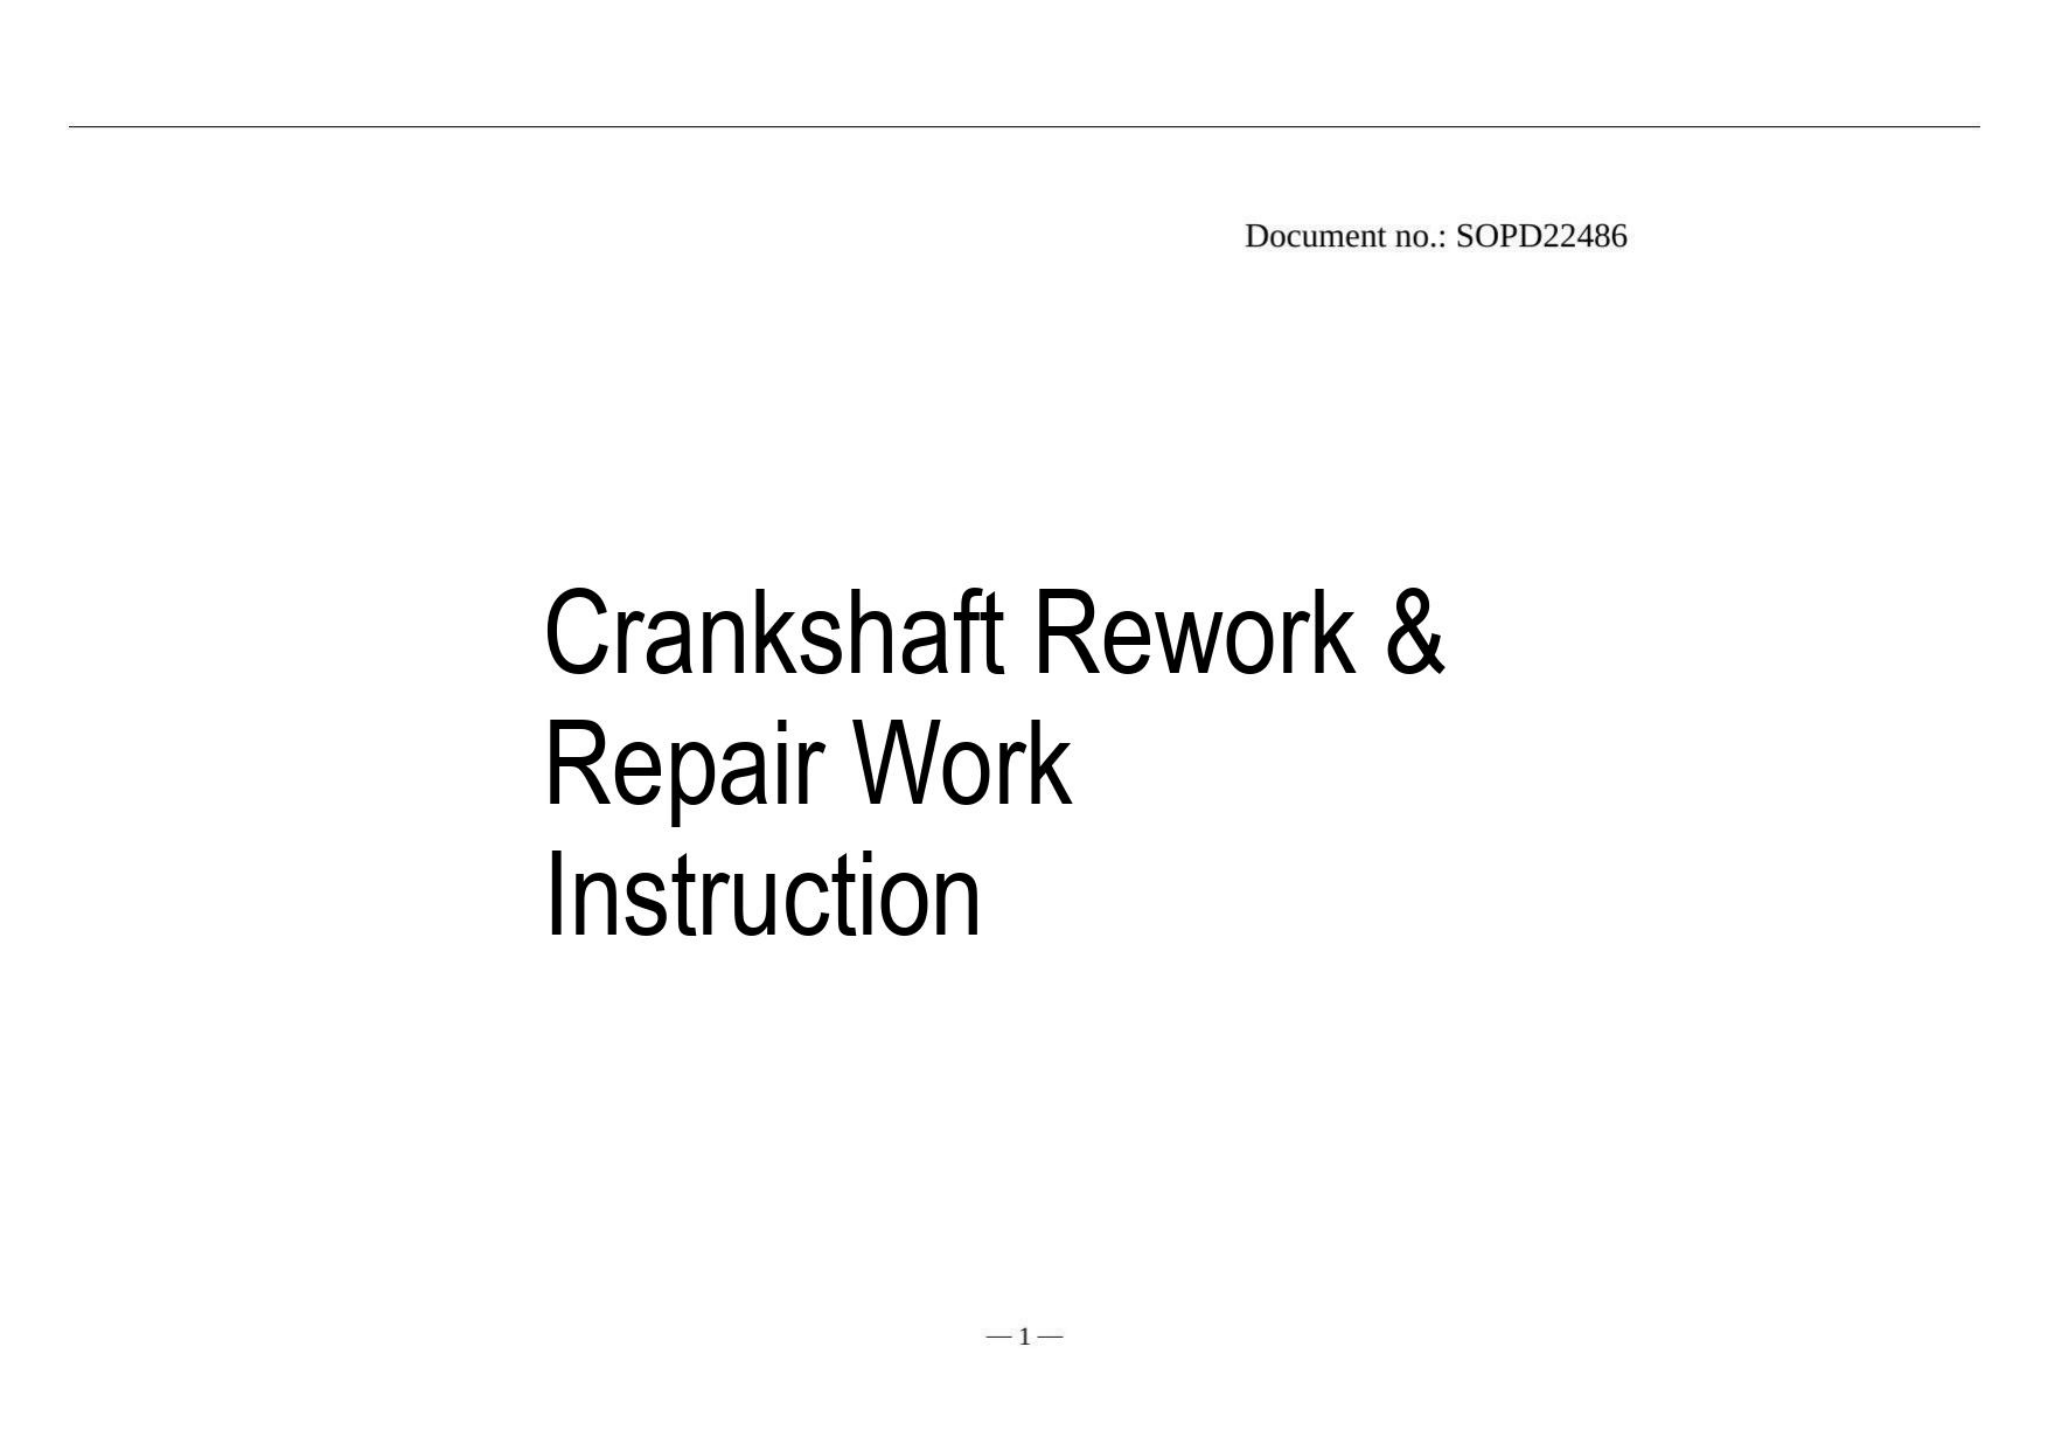Document no.: SOPD22486

Crankshaft Rework & Repair Work Instruction

—1—
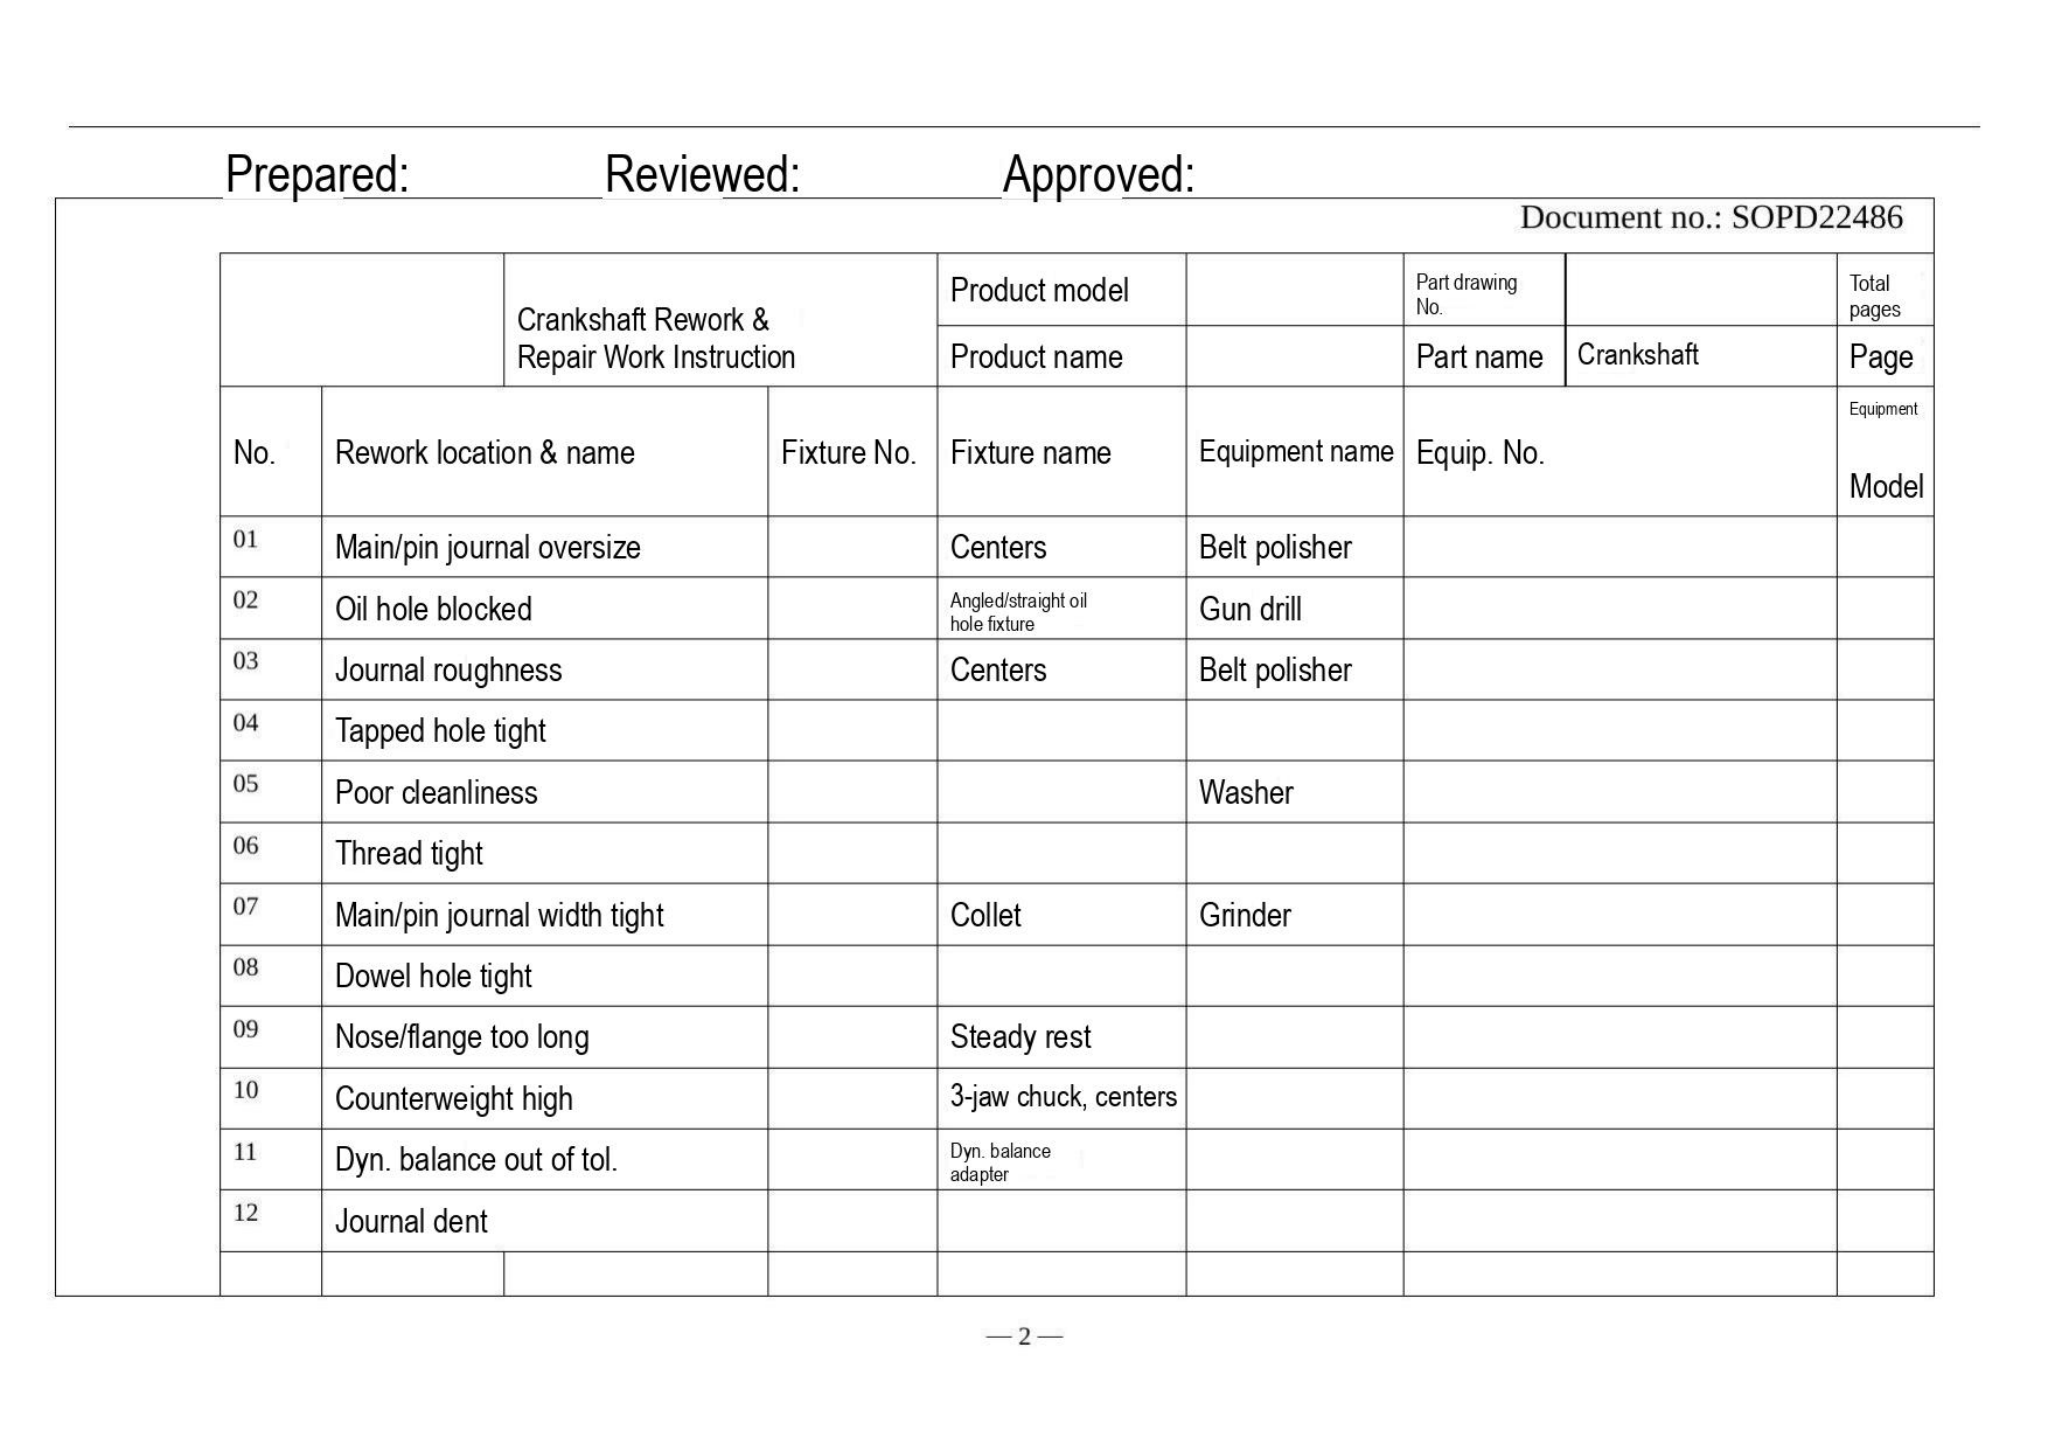Prepared: Reviewed: Approved:

Document no.: SOPD22486

| | Crankshaft Rework & Repair Work Instruction | Product model | | Part drawing No. | | Total pages |
|---|---|---|---|---|---|---|
| | | Product name | | Part name | Crankshaft | Page |

| No. | Rework location & name | Fixture No. | Fixture name | Equipment name | Equip. No. | Equipment Model |
|---|---|---|---|---|---|---|
| 01 | Main/pin journal oversize | | Centers | Belt polisher | | |
| 02 | Oil hole blocked | | Angled/straight oil hole fixture | Gun drill | | |
| 03 | Journal roughness | | Centers | Belt polisher | | |
| 04 | Tapped hole tight | | | | | |
| 05 | Poor cleanliness | | | Washer | | |
| 06 | Thread tight | | | | | |
| 07 | Main/pin journal width tight | | Collet | Grinder | | |
| 08 | Dowel hole tight | | | | | |
| 09 | Nose/flange too long | | Steady rest | | | |
| 10 | Counterweight high | | 3-jaw chuck, centers | | | |
| 11 | Dyn. balance out of tol. | | Dyn. balance adapter | | | |
| 12 | Journal dent | | | | | |
| | | | | | | |

—2—
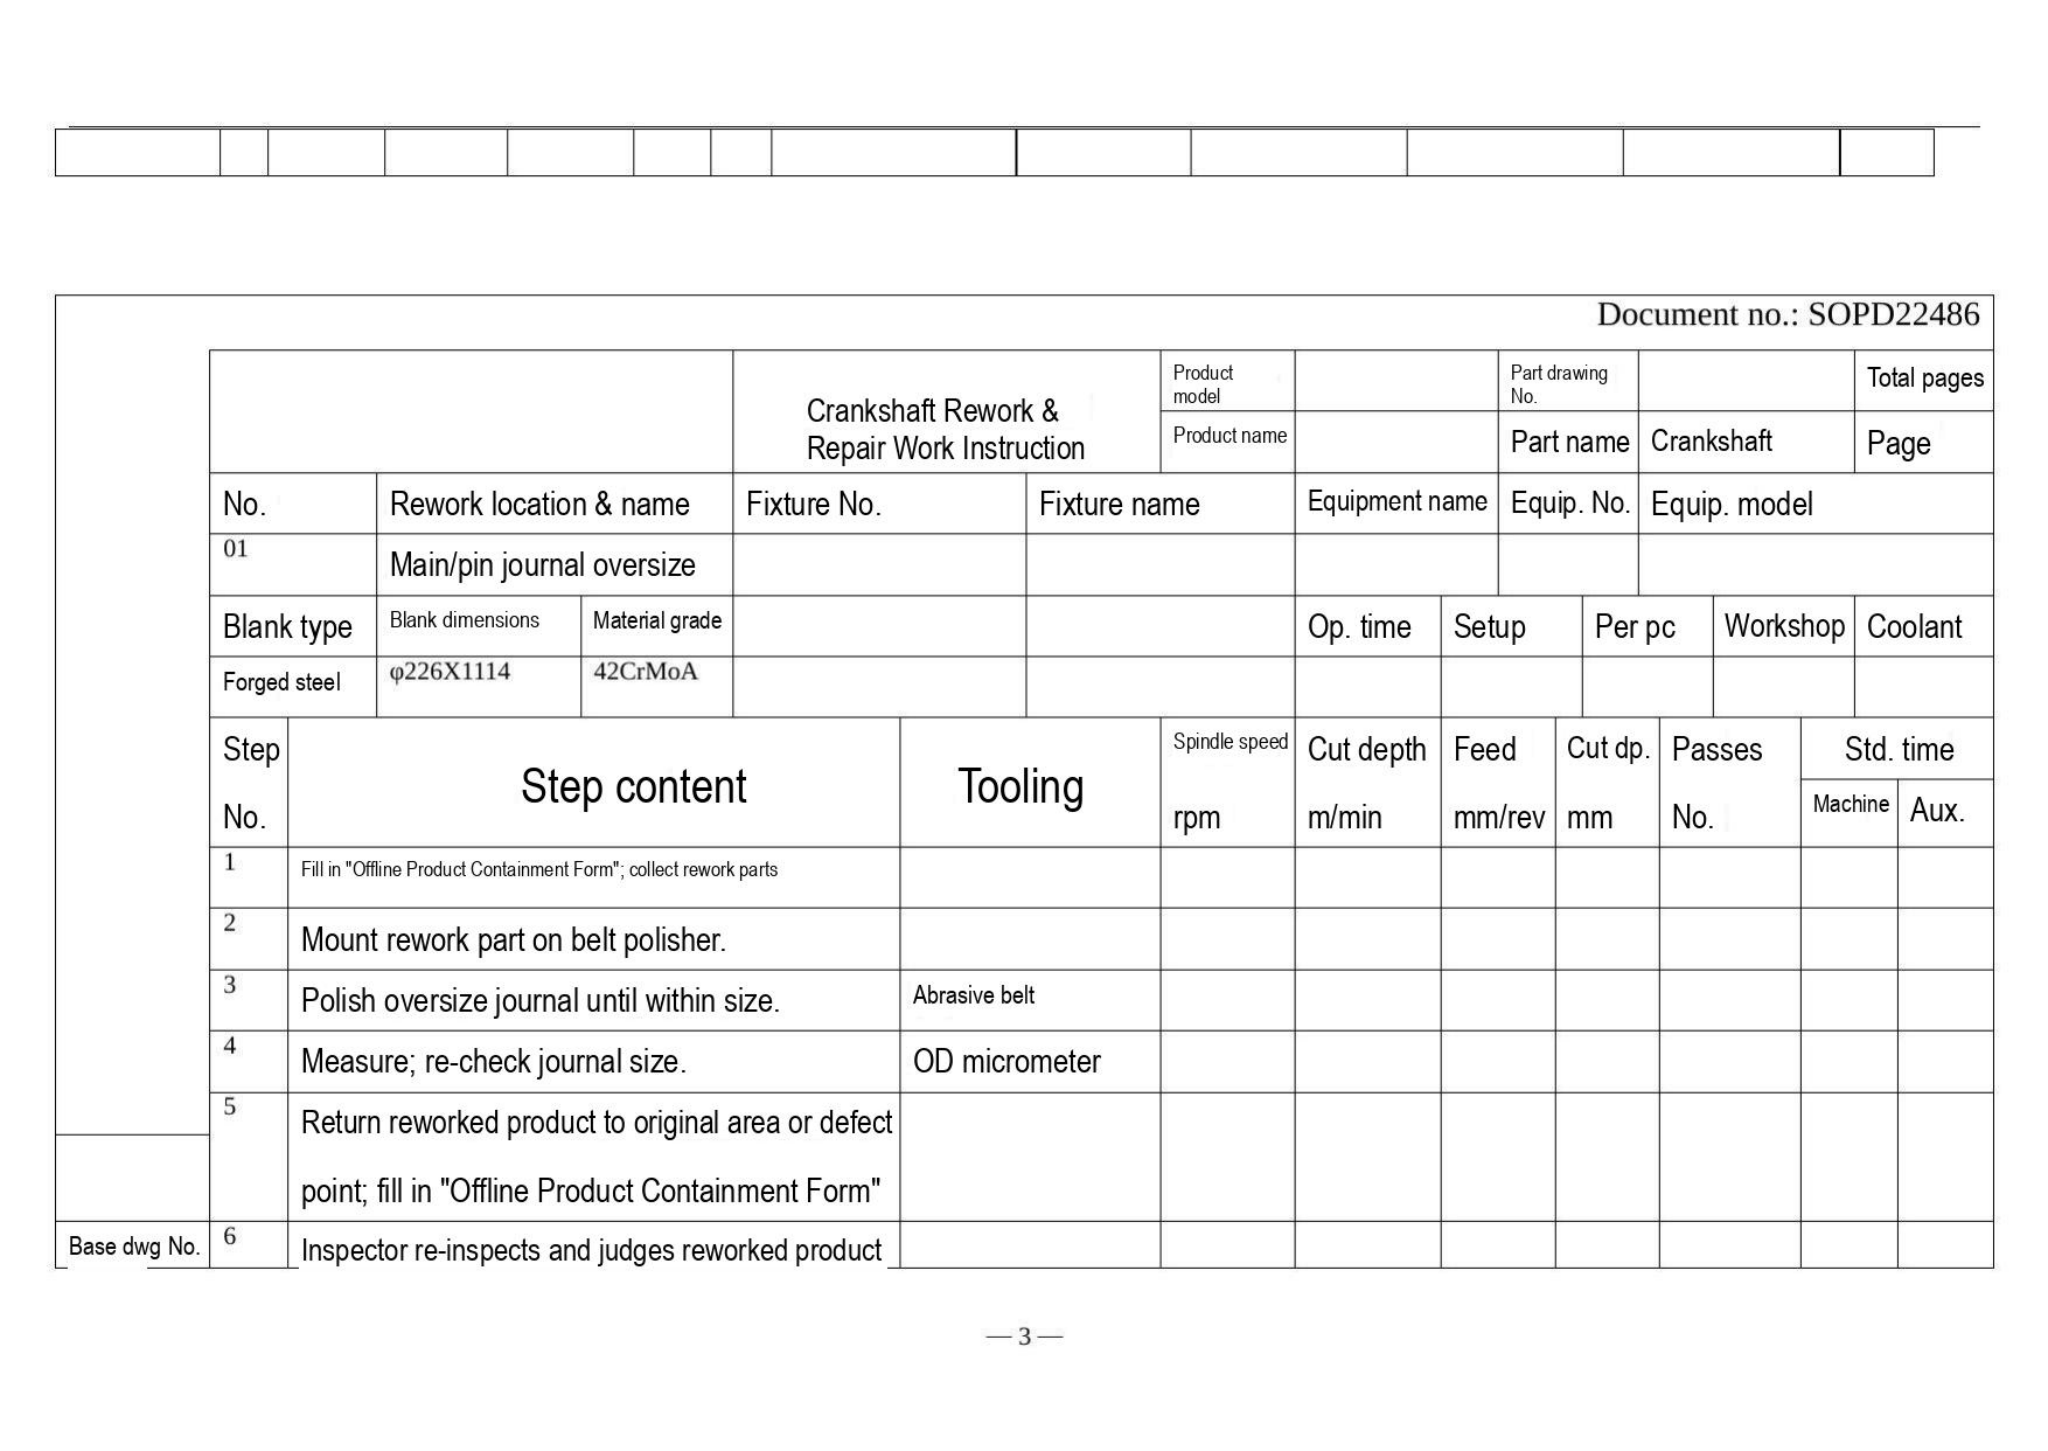Document no.: SOPD22486

| | Crankshaft Rework & Repair Work Instruction | Product model | | Part drawing No. | | Total pages |
|---|---|---|---|---|---|---|
| | | Product name | | Part name | Crankshaft | Page |

| No. | Rework location & name | Fixture No. | Fixture name | Equipment name | Equip. No. | Equip. model |
|---|---|---|---|---|---|---|
| 01 | Main/pin journal oversize | | | | | |

| Blank type | Blank dimensions | Material grade | | | Op. time | Setup | Per pc | Workshop | Coolant |
|---|---|---|---|---|---|---|---|---|---|
| Forged steel | φ226X1114 | 42CrMoA | | | | | | | |

| Step No. | Step content | Tooling | Spindle speed rpm | Cut depth m/min | Feed mm/rev | Cut dp. mm | Passes No. | Std. time Machine | Std. time Aux. |
|---|---|---|---|---|---|---|---|---|---|
| 1 | Fill in "Offline Product Containment Form"; collect rework parts | | | | | | | | |
| 2 | Mount rework part on belt polisher. | | | | | | | | |
| 3 | Polish oversize journal until within size. | Abrasive belt | | | | | | | |
| 4 | Measure; re-check journal size. | OD micrometer | | | | | | | |
| 5 | Return reworked product to original area or defect point; fill in "Offline Product Containment Form" | | | | | | | | |
| 6 | Inspector re-inspects and judges reworked product | | | | | | | | |

Base dwg No.

— 3 —
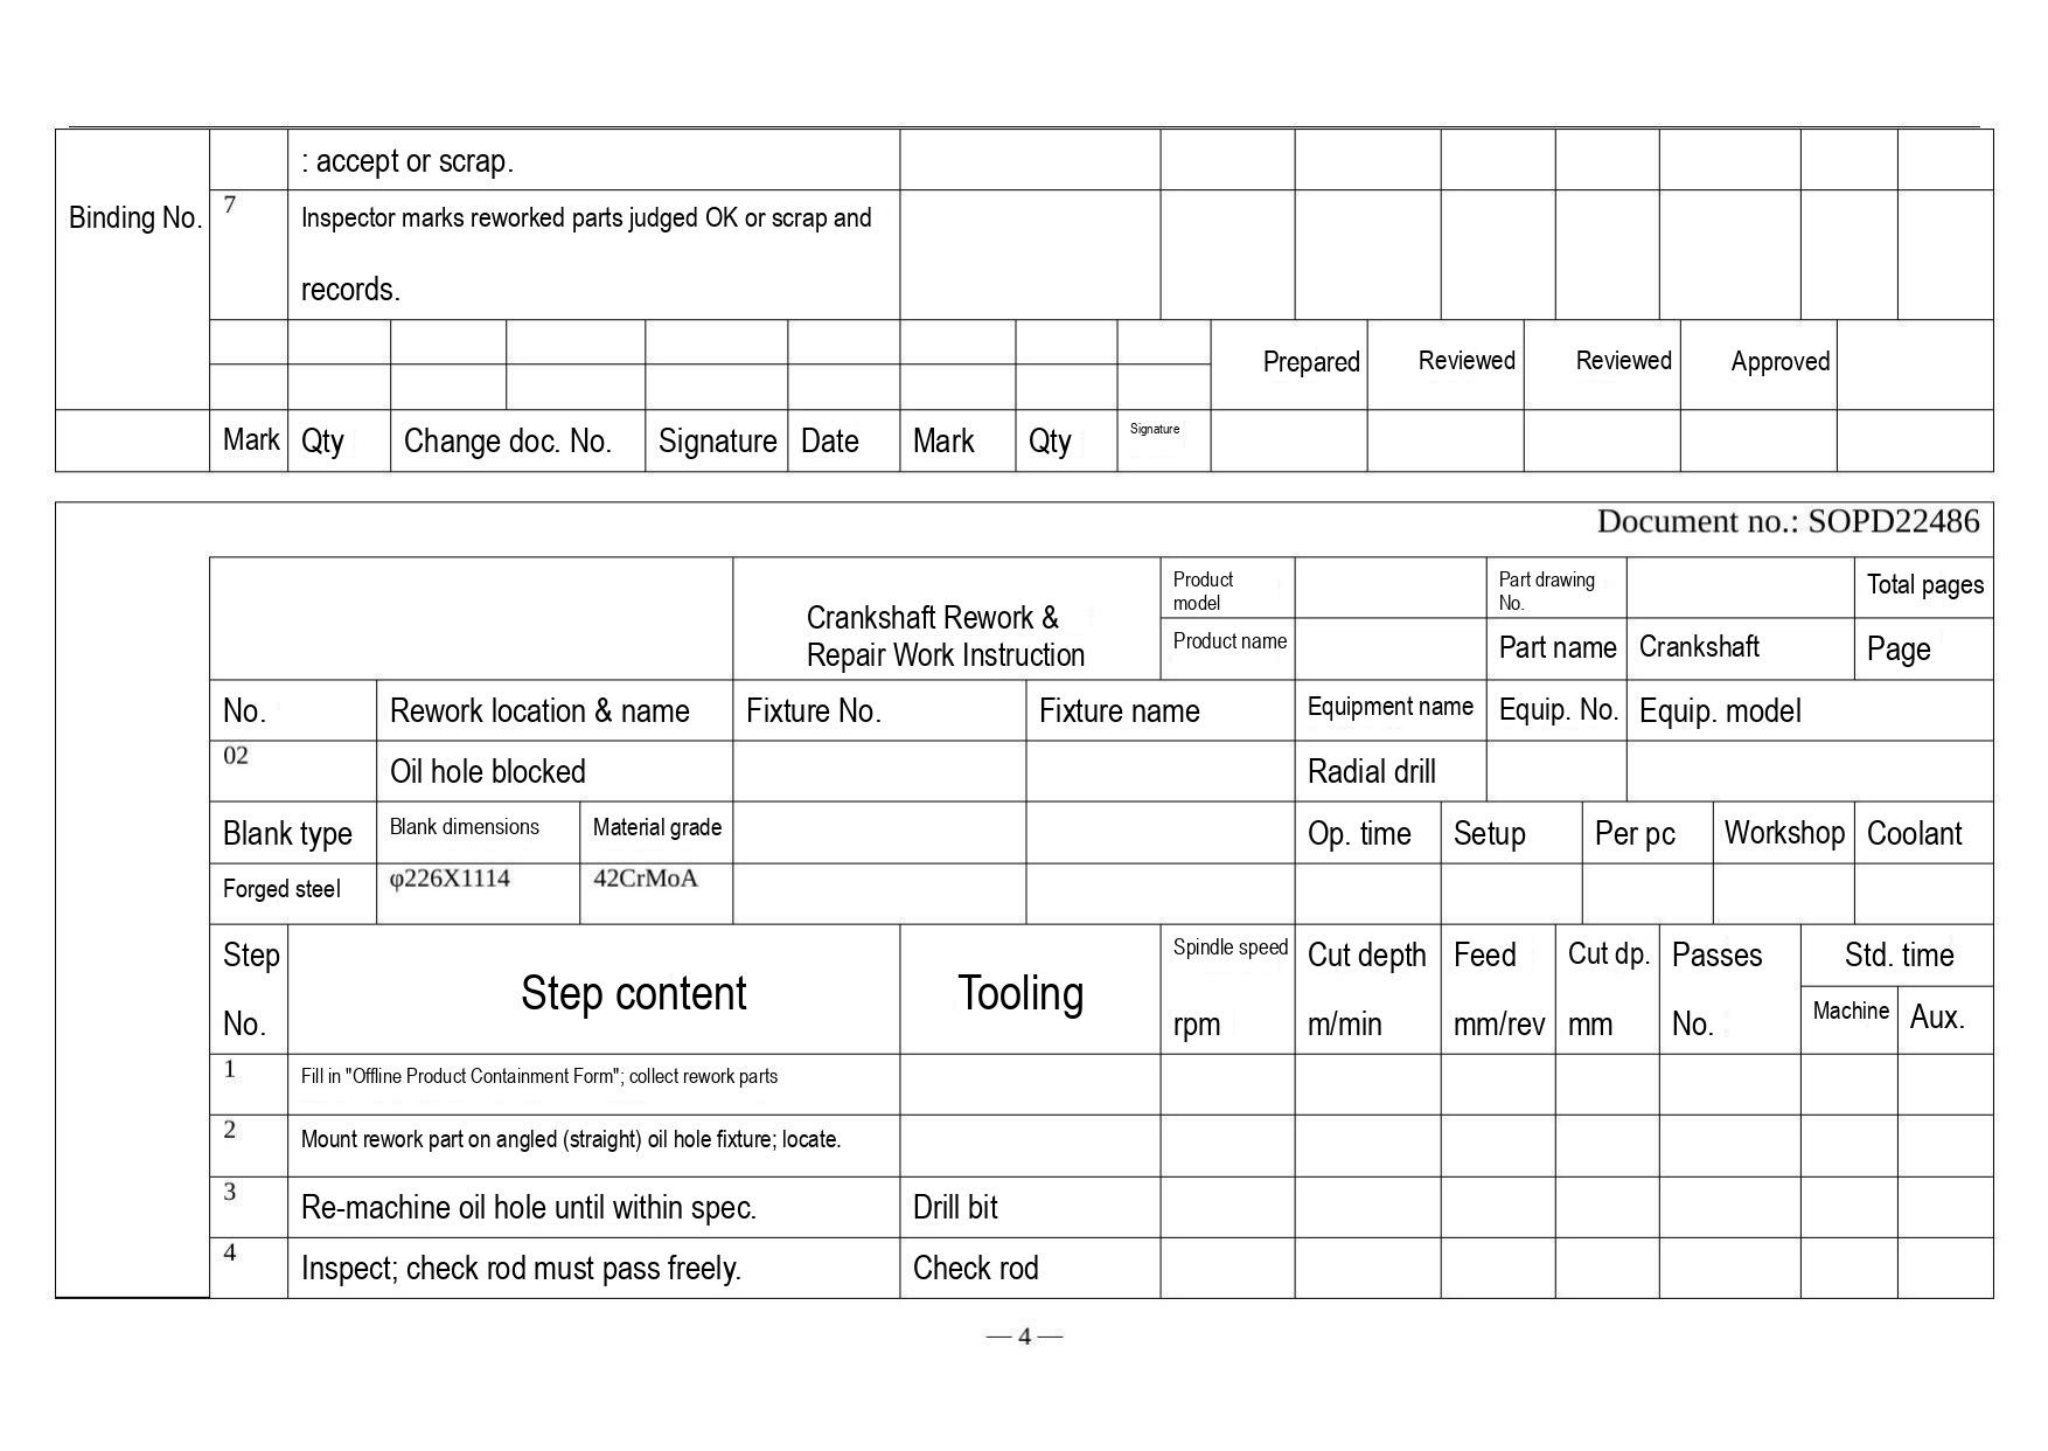| Binding No. | | : accept or scrap. | | | | | | | | |
|---|---|---|---|---|---|---|---|---|---|---|
| | 7 | Inspector marks reworked parts judged OK or scrap and records. | | | | | | | | |

| | | | | | | | | Prepared | Reviewed | Reviewed | Approved | |
|---|---|---|---|---|---|---|---|---|---|---|---|---|
| | | | | | | | | | | | | |
| Mark | Qty | Change doc. No. | Signature | Date | Mark | Qty | Signature | | | | | |

Document no.: SOPD22486

| | Crankshaft Rework & Repair Work Instruction | Product model | | Part drawing No. | | Total pages |
|---|---|---|---|---|---|---|
| | | Product name | | Part name | Crankshaft | Page |

| No. | Rework location & name | Fixture No. | Fixture name | Equipment name | Equip. No. | Equip. model |
|---|---|---|---|---|---|---|
| 02 | Oil hole blocked | | | Radial drill | | |

| Blank type | Blank dimensions | Material grade | | | Op. time | Setup | Per pc | Workshop | Coolant |
|---|---|---|---|---|---|---|---|---|---|
| Forged steel | φ226X1114 | 42CrMoA | | | | | | | |

| Step No. | Step content | Tooling | Spindle speed rpm | Cut depth m/min | Feed mm/rev | Cut dp. mm | Passes No. | Std. time Machine | Std. time Aux. |
|---|---|---|---|---|---|---|---|---|---|
| 1 | Fill in "Offline Product Containment Form"; collect rework parts | | | | | | | | |
| 2 | Mount rework part on angled (straight) oil hole fixture; locate. | | | | | | | | |
| 3 | Re-machine oil hole until within spec. | Drill bit | | | | | | | |
| 4 | Inspect; check rod must pass freely. | Check rod | | | | | | | |

—4—
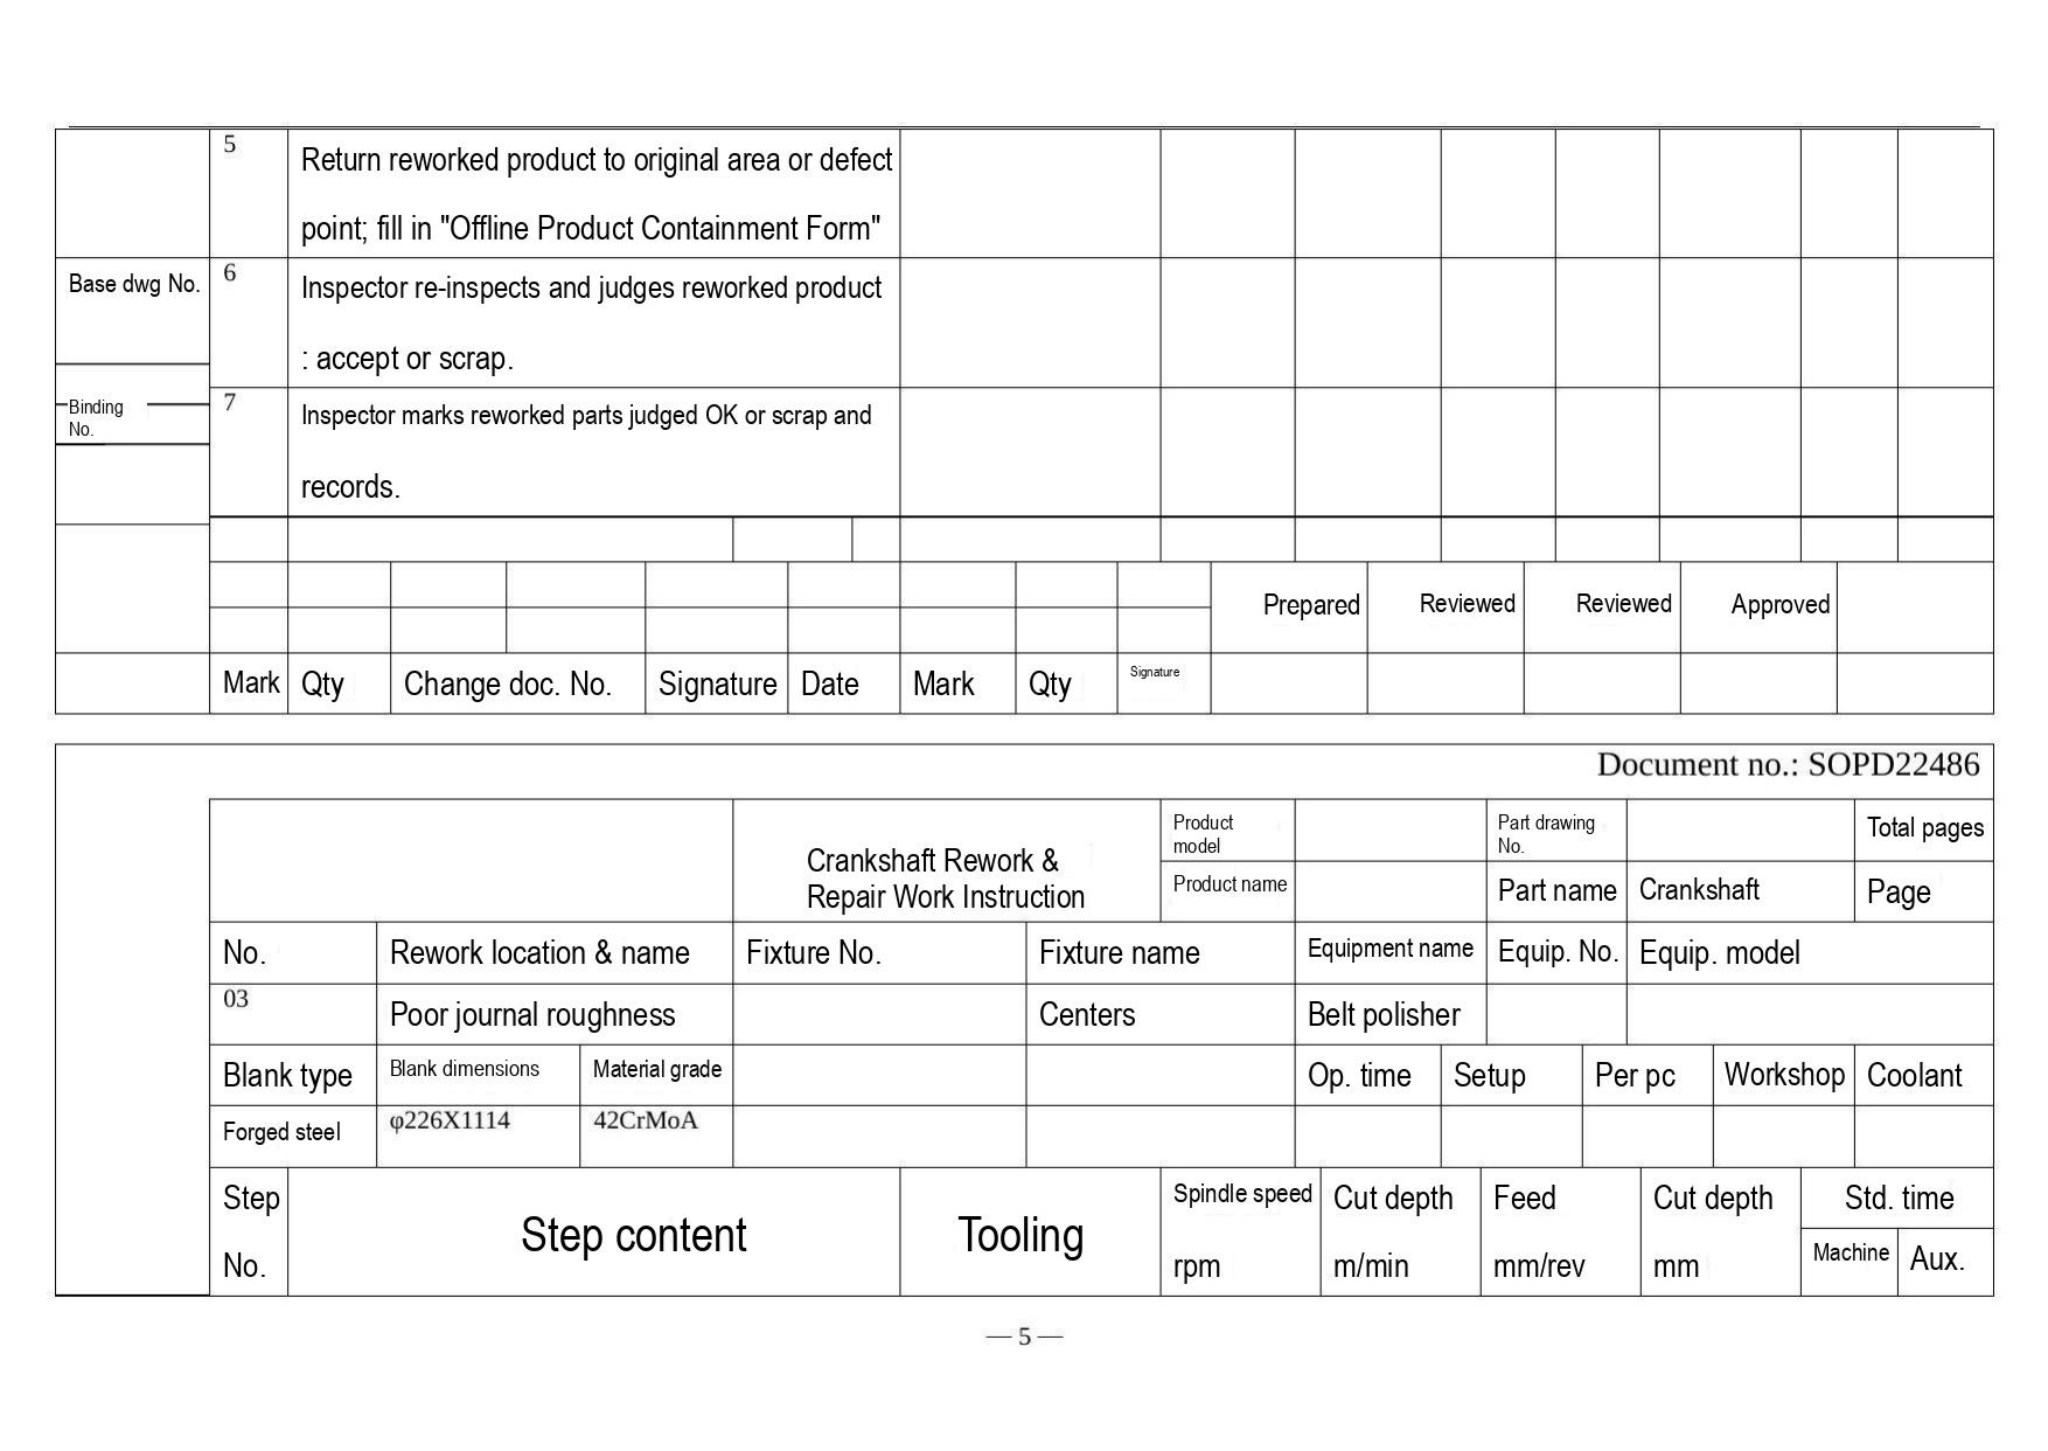| | | | | | | | | | | | | |
|---|---|---|---|---|---|---|---|---|---|---|---|---|
| | 5 | Return reworked product to original area or defect point; fill in "Offline Product Containment Form" | | | | | | | | | | |
| Base dwg No. | 6 | Inspector re-inspects and judges reworked product : accept or scrap. | | | | | | | | | | |
| Binding No. | 7 | Inspector marks reworked parts judged OK or scrap and records. | | | | | | | | | | |

| | | | | | | | | | | | | |
|---|---|---|---|---|---|---|---|---|---|---|---|---|
| | | | | | | | | Prepared | Reviewed | Reviewed | Approved | |
| | | | | | | | | | | | | |
| Mark | Qty | Change doc. No. | Signature | Date | Mark | Qty | Signature | | | | | |

Document no.: SOPD22486

| | Crankshaft Rework & Repair Work Instruction | Product model | | Part drawing No. | | Total pages |
|---|---|---|---|---|---|---|
| | | Product name | | Part name | Crankshaft | Page |

| No. | Rework location & name | Fixture No. | Fixture name | Equipment name | Equip. No. | Equip. model |
|---|---|---|---|---|---|---|
| 03 | Poor journal roughness | | Centers | Belt polisher | | |

| Blank type | Blank dimensions | Material grade | | | Op. time | Setup | Per pc | Workshop | Coolant |
|---|---|---|---|---|---|---|---|---|---|
| Forged steel | φ226X1114 | 42CrMoA | | | | | | | |

| Step No. | Step content | Tooling | Spindle speed rpm | Cut depth m/min | Feed mm/rev | Cut depth mm | Std. time Machine | Std. time Aux. |
|---|---|---|---|---|---|---|---|---|

—5—
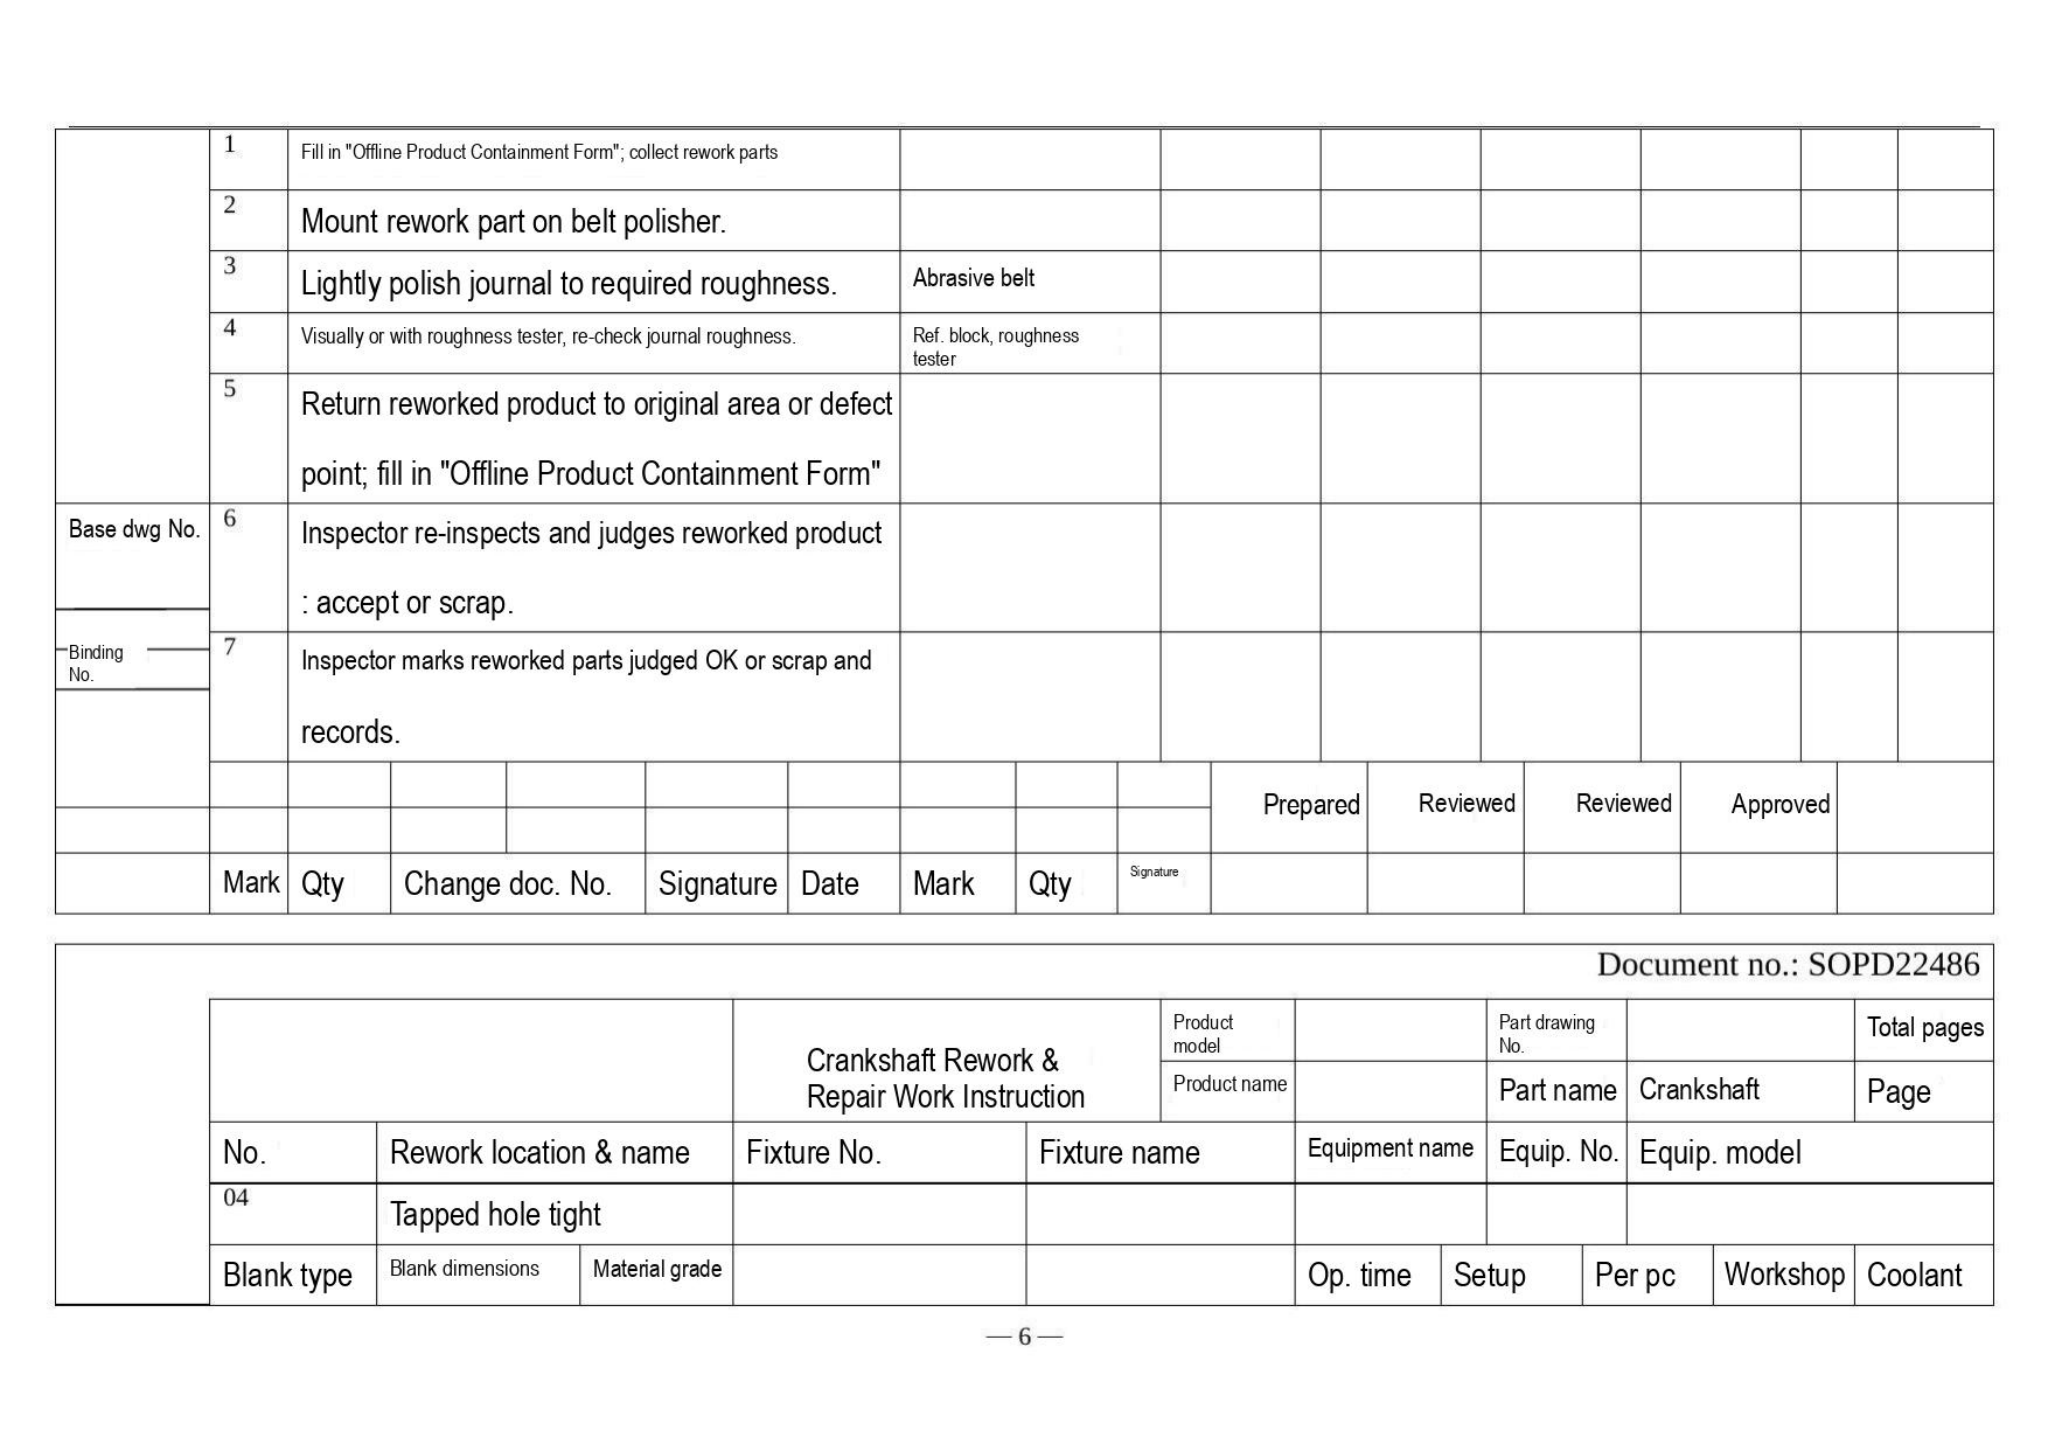| 1 | Fill in "Offline Product Containment Form"; collect rework parts | | | | | | | |
|---|---|---|---|---|---|---|---|---|
| 2 | Mount rework part on belt polisher. | | | | | | | |
| 3 | Lightly polish journal to required roughness. | Abrasive belt | | | | | | |
| 4 | Visually or with roughness tester, re-check journal roughness. | Ref. block, roughness tester | | | | | | |
| 5 | Return reworked product to original area or defect point; fill in "Offline Product Containment Form" | | | | | | | |
| 6 | Inspector re-inspects and judges reworked product : accept or scrap. | | | | | | | |
| 7 | Inspector marks reworked parts judged OK or scrap and records. | | | | | | | |

Base dwg No.

Binding No.

| | | | | | | | | Prepared | Reviewed | Reviewed | Approved | |
|---|---|---|---|---|---|---|---|---|---|---|---|---|
| | | | | | | | | | | | | |
| Mark | Qty | Change doc. No. | Signature | Date | Mark | Qty | Signature | | | | | |

Document no.: SOPD22486

| | Crankshaft Rework & Repair Work Instruction | Product model | | Part drawing No. | | Total pages |
|---|---|---|---|---|---|---|
| | | Product name | | Part name | Crankshaft | Page |

| No. | Rework location & name | Fixture No. | Fixture name | Equipment name | Equip. No. | Equip. model |
|---|---|---|---|---|---|---|
| 04 | Tapped hole tight | | | | | |

| Blank type | Blank dimensions | Material grade | | | Op. time | Setup | Per pc | Workshop | Coolant |
|---|---|---|---|---|---|---|---|---|---|

—6—
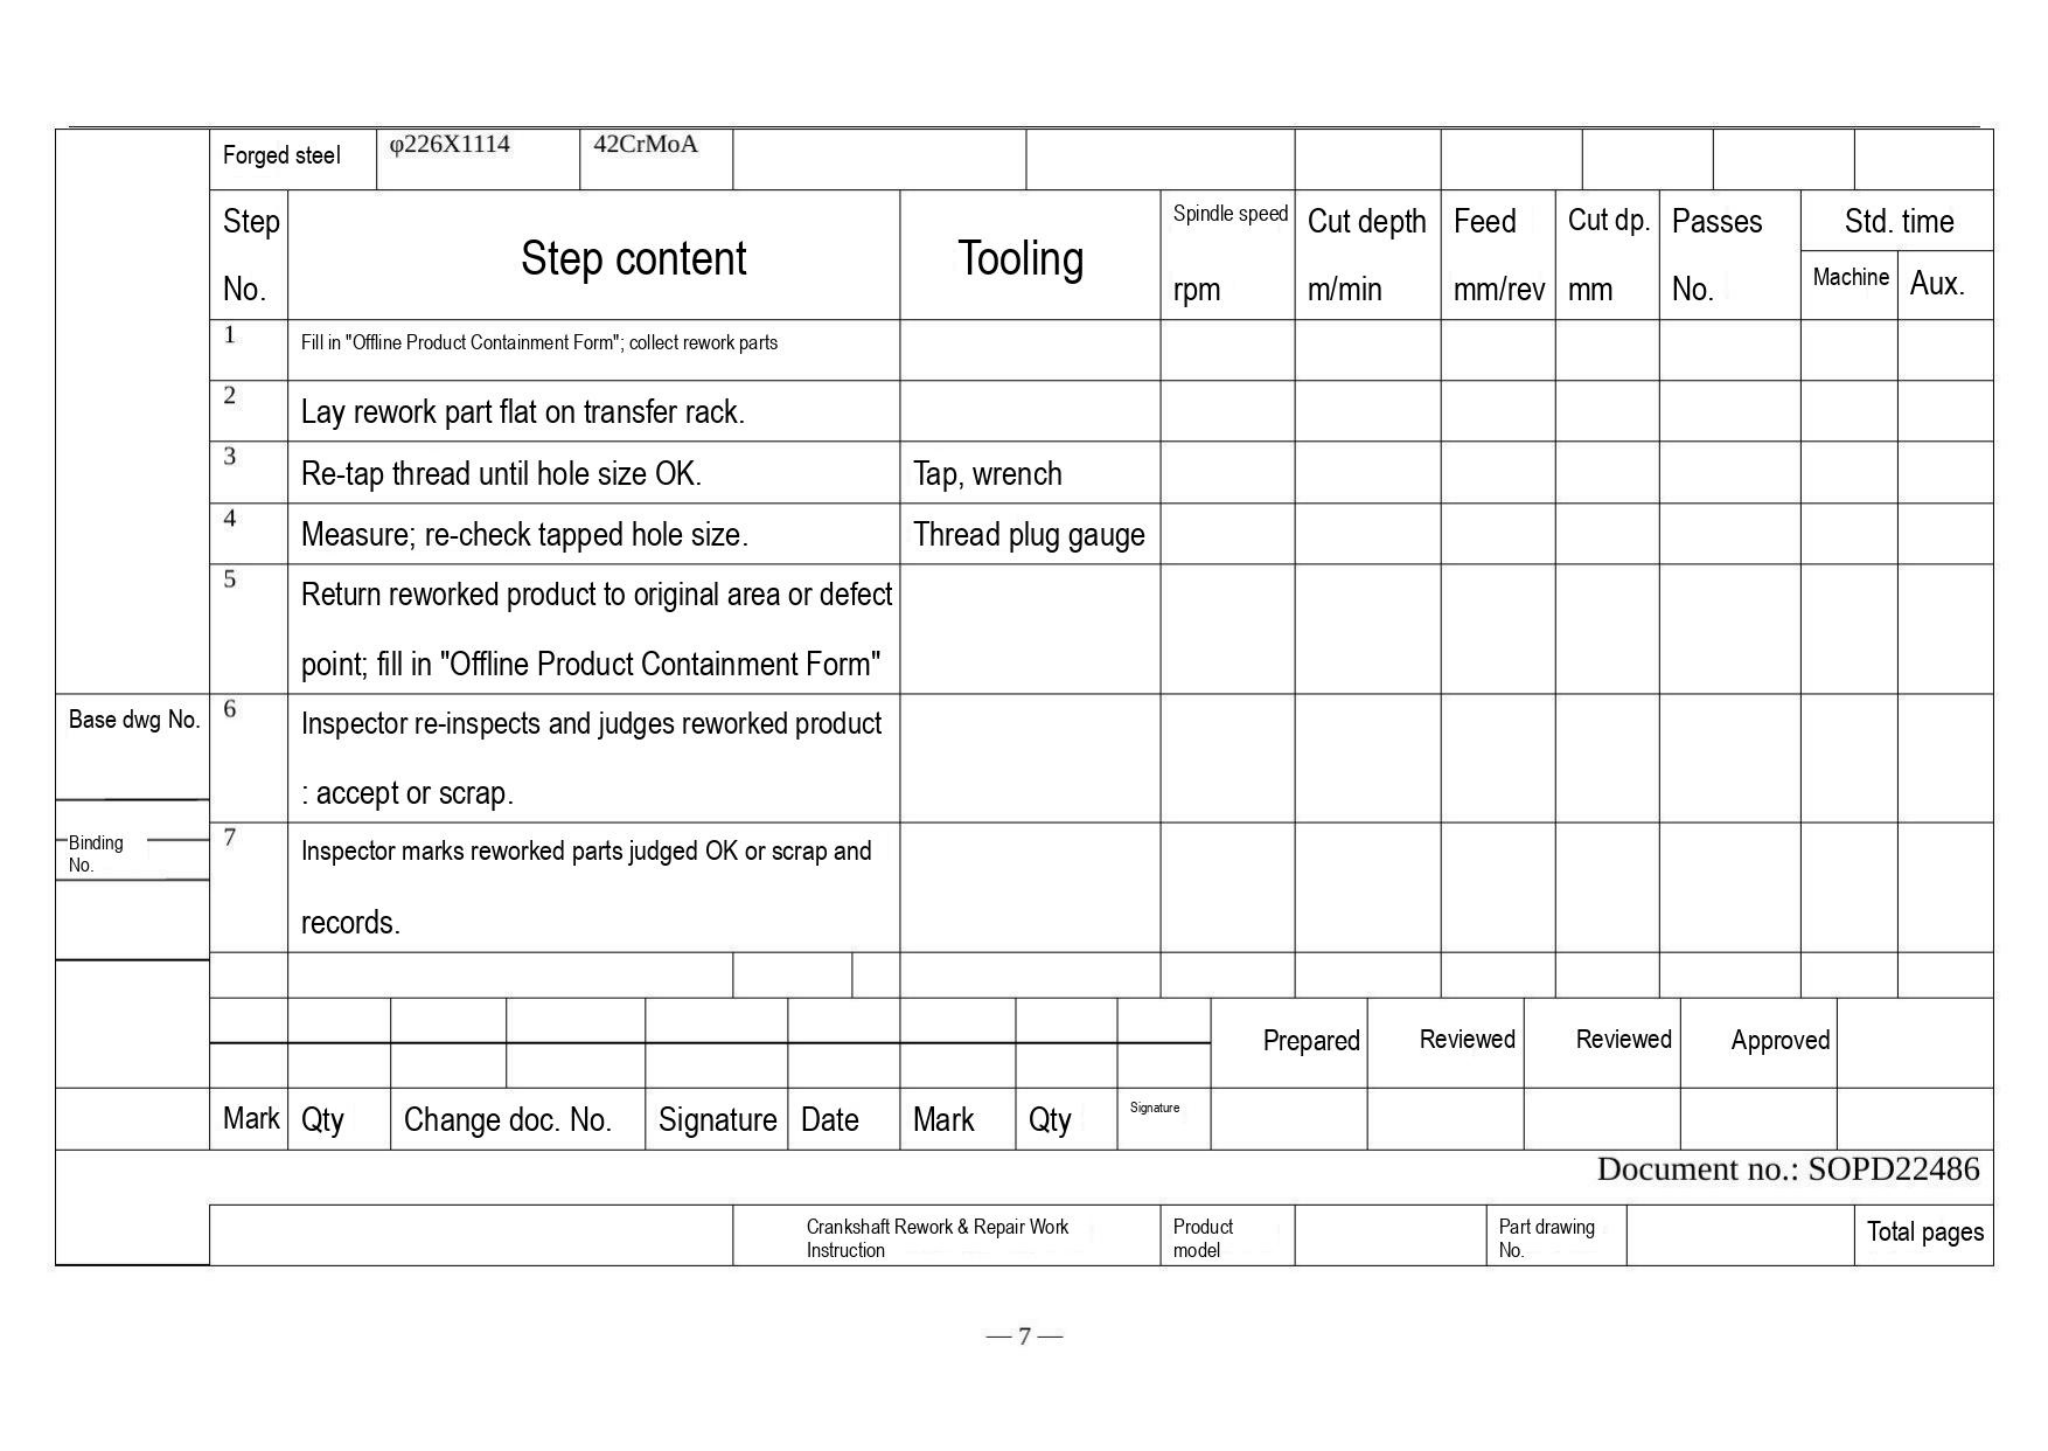| Forged steel | φ226X1114 | 42CrMoA | | | | | | | | |
|---|---|---|---|---|---|---|---|---|---|---|

| Step No. | Step content | Tooling | Spindle speed rpm | Cut depth m/min | Feed mm/rev | Cut dp. mm | Passes No. | Std. time Machine | Std. time Aux. |
|---|---|---|---|---|---|---|---|---|---|
| 1 | Fill in "Offline Product Containment Form"; collect rework parts | | | | | | | | |
| 2 | Lay rework part flat on transfer rack. | | | | | | | | |
| 3 | Re-tap thread until hole size OK. | Tap, wrench | | | | | | | |
| 4 | Measure; re-check tapped hole size. | Thread plug gauge | | | | | | | |
| 5 | Return reworked product to original area or defect point; fill in "Offline Product Containment Form" | | | | | | | | |
| 6 | Inspector re-inspects and judges reworked product : accept or scrap. | | | | | | | | |
| 7 | Inspector marks reworked parts judged OK or scrap and records. | | | | | | | | |

Base dwg No.

Binding No.

| Mark | Qty | Change doc. No. | Signature | Date | Mark | Qty | Signature | Prepared | Reviewed | Reviewed | Approved |
|---|---|---|---|---|---|---|---|---|---|---|---|

Document no.: SOPD22486

| | Crankshaft Rework & Repair Work Instruction | Product model | | Part drawing No. | | Total pages |
|---|---|---|---|---|---|---|

— 7 —